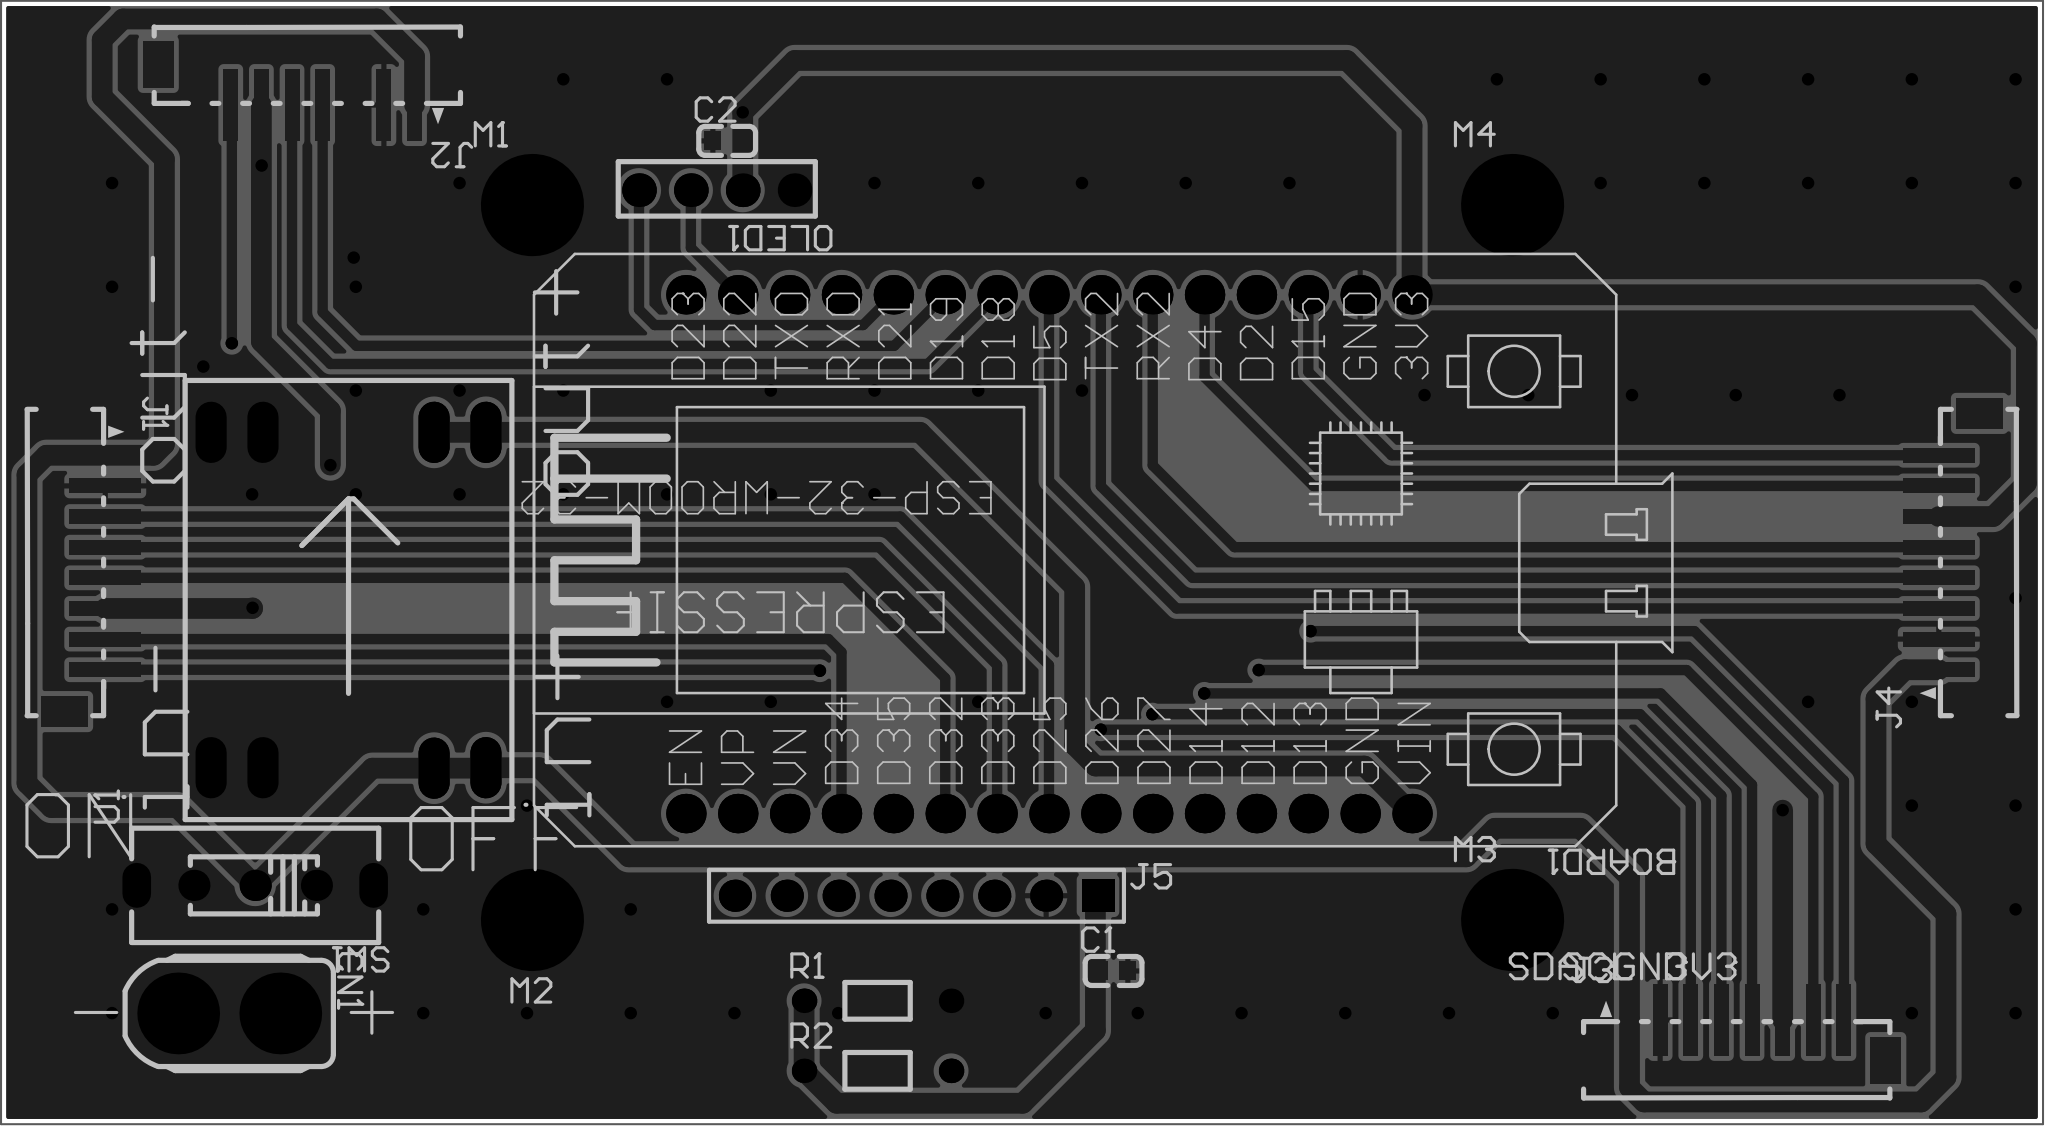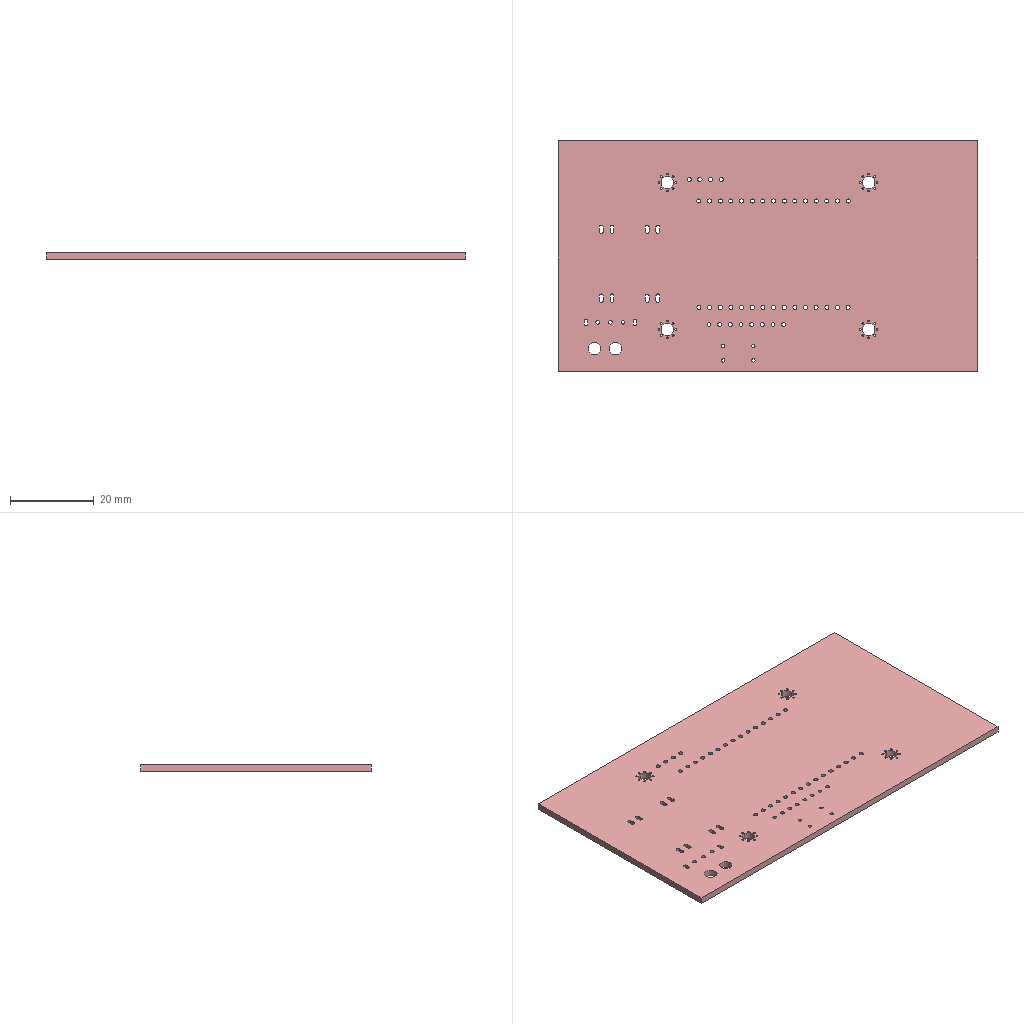Circuit board layout | Altium Designer | box 100 x 55 x 1.6 mm
Layer stack:
# Altium Designer layer stack of  (unit mm; dielectric type: 0 none, 1 core, 2 prepreg, 3 surface material)
index,name,kind,layer,copper_thickness_mm,dielectric_type,dielectric_thickness_mm,dielectric_material,dielectric_constant
0,Top Paste Mask Layer,other,,,,,,
1,Top Silkscreen Layer,other,,,,,,
2,Top Solder Mask Layer,dielectric,,,3,0.01,,3.3
3,Top Layer,copper,Top Layer,0.035,,,,
4,Dielectric1,dielectric,,,3,1.51,FR4,4.5
5,Bottom Layer,copper,Bottom Layer,0.035,,,,
6,Bottom Solder Mask Layer,dielectric,,,3,0.01,,3.3
7,Bottom Silkscreen Layer,other,,,,,,
8,Bottom Paste Mask Layer,other,,,,,,
# drill layer pairs: low layer,high layer
drill_pair,Top Layer,Bottom Layer
Part placement:
Designator,Comment,Layer,Footprint,Center-X(mm),Center-Y(mm),Rotation
M1,M3,TopLayer,M3,102.327,121.2,0
M2,M3,TopLayer,M3,102.327,86.2,0
M3,M3,TopLayer,M3,150.327,86.2,0
M4,M3,TopLayer,M3,150.327,121.2,0
U1,5v_buck,TopLayer,5V_BUCK,93.345,101.852,90
BOARD1,ESP32DEVKITV1 COPY,TopLayer,ESP32-DEVKITV1,127.647,104.108,180
SW1,SS-12F44-G6,TopLayer,SW-TH_SS-12F44-GX,88.773,87.893,180
CN1,XT30UPB-F,TopLayer,XT30,87.503,81.623,270
J5,HDR-M-2.54_1x8,TopLayer,HDR-M-2.54_1X8,121.158,87.385,180
J2,zh1.5-8p,TopLayer,ZH1.5-8P,91.327,127.096,180
J1,zh1.5-8p,TopLayer,ZH1.5-8P,80.431,103.7,270
J4,zh1.5-8p,TopLayer,ZH1.5-8P,172.223,103.7,90
J3,zh1.5-8p,TopLayer,ZH1.5-8P,161.327,80.304,0
OLED1,0.96OLED_4P_MODULE_JX,TopLayer,0.96OLED_4P,111.379,121.929,180
C1,100nF,TopLayer,C0603,130.81,83.702,0
C2,100nF,TopLayer,C0603,111.887,124.342,0
R1,4.7kΩ,TopLayer,Res_1/8W,119.253,82.241,0
R2,4.7kΩ,TopLayer,Res_1/8W,119.253,78.812,0
Pad and via stacks:
# Altium Designer via and pad stacks of  (unit mm). Each distinct definition once, with the count of objects using it.
# via: kind,start_layer,end_layer,hole_mm,diameter_mm,mode(0 simple;1 top-mid-bottom;2 full stack),diameter_per_layer,count,example_net
# pad: kind,layer,hole_mm,hole_type(0 round;1 square;2 slot),plating,top_size,top_shape(1 round;2 rect;3 octagon;9 rounded rect),mid_size,bottom_size,mode,footprint,size_per_layer,count,example
pad,Multi-Layer,0.4,2,plated,0.6x0.6,1,0.6x0.6,0.6x0.6,0,M3,,32,M1.1
pad,Multi-Layer,3,2,plated,5x5,1,5x5,5x5,0,M3,,4,M1.1
pad,Multi-Layer,0.9,2,plated,3x1.524,1,3x1.524,3x1.524,0,5V_BUCK,,8,U1.4
pad,Multi-Layer,0.9997,2,plated,1.93x1.93,1,1.93x1.93,1.93x1.93,0,ESP32-DEVKITV1,,30,BOARD1.3V3
pad,Multi-Layer,0.9144,0,plated,1.524x1.524,1,1.524x1.524,1.524x1.524,0,SW-TH_SS-12F44-GX,,3,SW1.1
pad,Multi-Layer,0.8,2,plated,2.2x1.4,1,2.2x1.4,2.2x1.4,0,SW-TH_SS-12F44-GX,,2,SW1.4
pad,Multi-Layer,3,0,plated,4x4,1,4x4,4x4,0,XT30,,2,CN1.1
pad,Multi-Layer,0.889,0,plated,1.575x1.575,2,1.575x1.575,1.575x1.575,0,HDR-M-2.54_1X8,,1,J5.1
pad,Multi-Layer,0.889,0,plated,1.575x1.575,1,1.575x1.575,1.575x1.575,0,HDR-M-2.54_1X8,,7,J5.2
pad,Multi-Layer,1,0,plated,1.65x1.65,1,1.65x1.65,1.65x1.65,0,0.96OLED_4P,,4,OLED1.4
pad,Multi-Layer,0.8001,0,plated,1.199x1.199,1,1.199x1.199,1.199x1.199,0,Res_1/8W,,4,R1.1
pad,Top Layer,0,0,plated,0.7x3.5,2,0.7x3.5,0.7x3.5,0,ZH1.5-8P,,32,J2.6
pad,Top Layer,0,0,plated,1.5x2.3,2,1.5x2.3,1.5x2.3,0,ZH1.5-8P,,8,J2.9
pad,Top Layer,0,0,plated,0.8x0.9,2,0.8x0.9,0.8x0.9,0,C0603,,4,C1.2
via,Top Layer,Bottom Layer,0.3048,0.61,0,,14,M3PWM
via,Top Layer,Bottom Layer,0.3048,0.6096,0,,69,GND
Copper pours:
name,layer,net,type(0 solid;1 hatched;2 none)
Bottom Layer-GND,Bottom Layer,GND,0
Top Layer-GND,Top Layer,GND,0
Design rules, without the lines most boards share:
# Altium Designer design rules of  (exported by Altium Designer, unit mm)
# columns: name | kind | enabled | priority | scope1 | scope2 | descriptor | typed fields (field=value)
copperThickness2oz | 0 | disabled | 1 | All | All | Clearance Constraint (Gap=6mil) (Disabled)(All),(All) | gap=0.1524
otherClearance | 52 | enabled | 1 | All | All | Hole To Hole Clearance (Gap=11.8mil) (All),(All) | gap=0.2997
viaSize | 11 | enabled | 1 | All | All | Routing Via (MinHoleWidth=11.8mil) (MaxHoleWidth=248mil) (PreferredHoleWidth=12mil) (MinWidth=19.7mil) (MaxWidth=393.7mil) (PreferedWidth=24mil) (All) | via_min_hole=0.2997 via_max_hole=6.299 via_preferred_diameter=0.6096 via_preferred_hole=0.3048